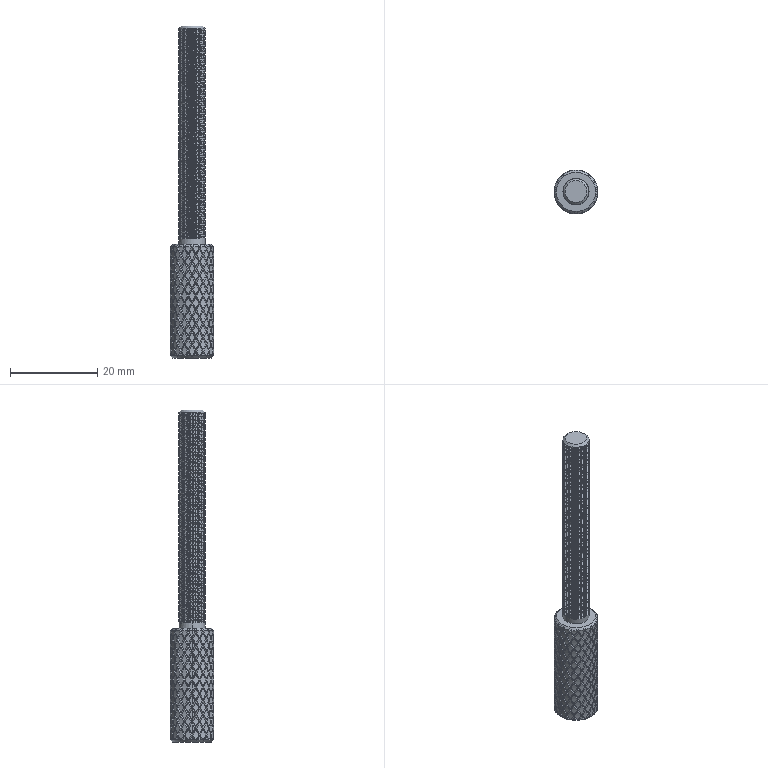Part | SolidWorks | features Chamfer 1, CirPattern 1, Extrusion 1, ICE 1, MirrorPattern 1, SweepCut 1, SweepThread 1 | 1 solid | 1857 faces | box 10 x 10.004 x 76 mm | volume 3336 mm3 | spline 1227 | cylinder 619 | cone 6 | plane 5 | commonest cylinder face diameters 10 x315 6 x304